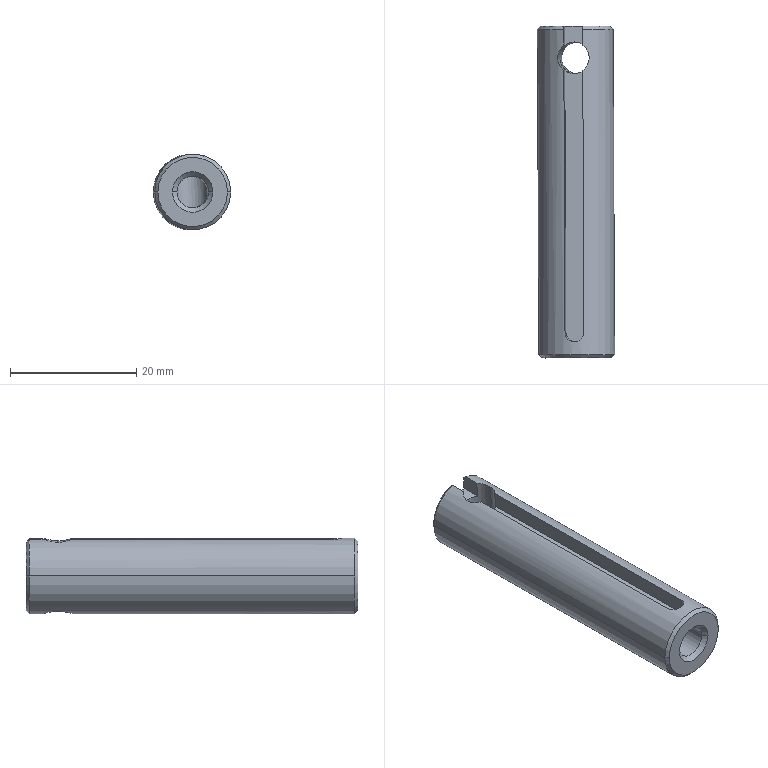Part | SolidWorks | features BaseBody 1 | 1 solid | 22 faces | box 12.224 x 52.547 x 12 mm | volume 4434 mm3 | plane 8 | cylinder 7 | cone 7 | commonest cylinder face diameters 5 x4 12 x2 3 x1
STEP:
#1=CARTESIAN_POINT('',(589.455,-135.542,110.117));
#2=VERTEX_POINT('',#1);
#3=CARTESIAN_POINT('',(585.292,-135.56,104.405));
#4=VERTEX_POINT('',#3);
#5=CARTESIAN_POINT('',(591.292,-135.534,104.405));
#6=DIRECTION('',(0.004352,-1.,-0.000000003));
#7=DIRECTION('',(1.,0.004352,0.));
#8=AXIS2_PLACEMENT_3D('',#5,#6,#7);
#9=CIRCLE('',#8,6.);
#10=EDGE_CURVE('',#2,#4,#9,.T.);
#11=ORIENTED_EDGE('',*,*,#10,.T.);
#12=CARTESIAN_POINT('',(585.516,-187.059,104.405));
#13=VERTEX_POINT('',#12);
#14=CARTESIAN_POINT('',(585.278,-132.435,104.405));
#15=DIRECTION('',(0.004352,-1.,-0.000000003));
#16=VECTOR('',#15,1000.);
#17=LINE('',#14,#16);
#18=EDGE_CURVE('',#4,#13,#17,.T.);
#19=ORIENTED_EDGE('',*,*,#18,.T.);
#20=CARTESIAN_POINT('',(597.516,-187.007,104.405));
#21=VERTEX_POINT('',#20);
#22=CARTESIAN_POINT('',(591.516,-187.033,104.405));
#23=DIRECTION('',(-0.004352,1.,0.000000003));
#24=DIRECTION('',(1.,0.004352,0.));
#25=AXIS2_PLACEMENT_3D('',#22,#23,#24);
#26=CIRCLE('',#25,6.);
#27=EDGE_CURVE('',#13,#21,#26,.T.);
#28=ORIENTED_EDGE('',*,*,#27,.T.);
#29=CARTESIAN_POINT('',(597.292,-135.507,104.405));
#30=VERTEX_POINT('',#29);
#31=CARTESIAN_POINT('',(597.278,-132.383,104.405));
#32=DIRECTION('',(0.004352,-1.,-0.000000003));
#33=VECTOR('',#32,1000.);
#34=LINE('',#31,#33);
#35=EDGE_CURVE('',#30,#21,#34,.T.);
#36=ORIENTED_EDGE('',*,*,#35,.F.);
#37=CARTESIAN_POINT('',(592.45,-135.529,110.292));
#38=VERTEX_POINT('',#37);
#39=CARTESIAN_POINT('',(591.292,-135.534,104.405));
#40=DIRECTION('',(0.004352,-1.,-0.000000003));
#41=DIRECTION('',(1.,0.004352,0.));
#42=AXIS2_PLACEMENT_3D('',#39,#40,#41);
#43=CIRCLE('',#42,6.);
#44=EDGE_CURVE('',#30,#38,#43,.T.);
#45=ORIENTED_EDGE('',*,*,#44,.T.);
#46=CARTESIAN_POINT('',(592.461,-138.029,110.292));
#47=VERTEX_POINT('',#46);
#48=CARTESIAN_POINT('',(592.436,-132.404,110.292));
#49=DIRECTION('',(0.004352,-1.,-0.000000003));
#50=VECTOR('',#49,1000.);
#51=LINE('',#48,#50);
#52=EDGE_CURVE('',#38,#47,#51,.T.);
#53=ORIENTED_EDGE('',*,*,#52,.T.);
#54=CARTESIAN_POINT('',(593.489,-140.035,109.996));
#55=VERTEX_POINT('',#54);
#56=CARTESIAN_POINT('',(592.461,-138.029,110.292));
#57=CARTESIAN_POINT('',(592.619,-138.145,110.261));
#58=CARTESIAN_POINT('',(592.761,-138.276,110.227));
#59=CARTESIAN_POINT('',(593.013,-138.569,110.158));
#60=CARTESIAN_POINT('',(593.124,-138.733,110.124));
#61=CARTESIAN_POINT('',(593.302,-139.077,110.065));
#62=CARTESIAN_POINT('',(593.371,-139.26,110.039));
#63=CARTESIAN_POINT('',(593.465,-139.644,110.005));
#64=CARTESIAN_POINT('',(593.489,-139.838,109.996));
#65=CARTESIAN_POINT('',(593.489,-140.035,109.996));
#66=B_SPLINE_CURVE_WITH_KNOTS('',3,(#56,#57,#58,#59,#60,#61,#62,#63,#64,#65),.UNSPECIFIED.,.F.,.F.,(4,2,2,2,4),(0.,0.000588,0.001176,0.001764,0.002352),.UNSPECIFIED.);
#67=EDGE_CURVE('',#47,#55,#66,.T.);
#68=ORIENTED_EDGE('',*,*,#67,.T.);
#69=CARTESIAN_POINT('',(592.478,-142.028,110.292));
#70=VERTEX_POINT('',#69);
#71=CARTESIAN_POINT('',(593.489,-140.035,109.996));
#72=CARTESIAN_POINT('',(593.489,-140.229,109.996));
#73=CARTESIAN_POINT('',(593.465,-140.426,110.006));
#74=CARTESIAN_POINT('',(593.373,-140.801,110.041));
#75=CARTESIAN_POINT('',(593.305,-140.984,110.066));
#76=CARTESIAN_POINT('',(593.042,-141.498,110.155));
#77=CARTESIAN_POINT('',(592.789,-141.796,110.231));
#78=CARTESIAN_POINT('',(592.478,-142.028,110.292));
#79=B_SPLINE_CURVE_WITH_KNOTS('',3,(#71,#72,#73,#74,#75,#76,#77,#78),.UNSPECIFIED.,.F.,.F.,(4,2,2,4),(0.002352,0.002933,0.003513,0.004674),.UNSPECIFIED.);
#80=EDGE_CURVE('',#55,#70,#79,.T.);
#81=ORIENTED_EDGE('',*,*,#80,.T.);
#82=CARTESIAN_POINT('',(592.659,-183.528,110.292));
#83=VERTEX_POINT('',#82);
#84=CARTESIAN_POINT('',(592.436,-132.404,110.292));
#85=DIRECTION('',(0.004352,-1.,-0.000000003));
#86=VECTOR('',#85,1000.);
#87=LINE('',#84,#86);
#88=EDGE_CURVE('',#70,#83,#87,.T.);
#89=ORIENTED_EDGE('',*,*,#88,.T.);
#90=CARTESIAN_POINT('',(589.664,-183.541,110.117));
#91=VERTEX_POINT('',#90);
#92=CARTESIAN_POINT('',(592.659,-183.528,110.292));
#93=CARTESIAN_POINT('',(592.659,-183.628,110.292));
#94=CARTESIAN_POINT('',(592.65,-183.725,110.294));
#95=CARTESIAN_POINT('',(592.612,-183.918,110.302));
#96=CARTESIAN_POINT('',(592.583,-184.013,110.307));
#97=CARTESIAN_POINT('',(592.508,-184.195,110.321));
#98=CARTESIAN_POINT('',(592.461,-184.281,110.328));
#99=CARTESIAN_POINT('',(592.352,-184.444,110.345));
#100=CARTESIAN_POINT('',(592.289,-184.521,110.354));
#101=CARTESIAN_POINT('',(592.081,-184.729,110.379));
#102=CARTESIAN_POINT('',(591.914,-184.841,110.394));
#103=CARTESIAN_POINT('',(591.553,-184.993,110.408));
#104=CARTESIAN_POINT('',(591.356,-185.034,110.406));
#105=CARTESIAN_POINT('',(591.058,-185.035,110.389));
#106=CARTESIAN_POINT('',(590.96,-185.026,110.381));
#107=CARTESIAN_POINT('',(590.769,-184.988,110.36));
#108=CARTESIAN_POINT('',(590.674,-184.96,110.348));
#109=CARTESIAN_POINT('',(590.493,-184.885,110.319));
#110=CARTESIAN_POINT('',(590.408,-184.839,110.304));
#111=CARTESIAN_POINT('',(590.246,-184.731,110.272));
#112=CARTESIAN_POINT('',(590.17,-184.669,110.255));
#113=CARTESIAN_POINT('',(589.965,-184.463,110.206));
#114=CARTESIAN_POINT('',(589.855,-184.297,110.174));
#115=CARTESIAN_POINT('',(589.705,-183.937,110.13));
#116=CARTESIAN_POINT('',(589.665,-183.74,110.117));
#117=CARTESIAN_POINT('',(589.664,-183.541,110.117));
#118=B_SPLINE_CURVE_WITH_KNOTS('',3,(#92,#93,#94,#95,#96,#97,#98,#99,#100,#101,#102,#103,#104,#105,#106,#107,#108,#109,#110,#111,#112,#113,#114,#115,#116,#117),.UNSPECIFIED.,.F.,.F.,(4,2,2,2,2,2,2,2,2,2,2,2,4),(0.,0.0002941,0.0005882,0.0008822,0.001176,0.001764,0.002353,0.002647,0.002941,0.003235,0.003529,0.004117,0.004705),.UNSPECIFIED.);
#119=EDGE_CURVE('',#83,#91,#118,.T.);
#120=ORIENTED_EDGE('',*,*,#119,.T.);
#121=CARTESIAN_POINT('',(589.484,-142.042,110.117));
#122=VERTEX_POINT('',#121);
#123=CARTESIAN_POINT('',(589.442,-132.417,110.117));
#124=DIRECTION('',(-0.004352,1.,0.000000003));
#125=VECTOR('',#124,1000.);
#126=LINE('',#123,#125);
#127=EDGE_CURVE('',#91,#122,#126,.T.);
#128=ORIENTED_EDGE('',*,*,#127,.T.);
#129=CARTESIAN_POINT('',(588.497,-140.035,109.704));
#130=VERTEX_POINT('',#129);
#131=CARTESIAN_POINT('',(589.484,-142.042,110.117));
#132=CARTESIAN_POINT('',(589.33,-141.925,110.068));
#133=CARTESIAN_POINT('',(589.193,-141.794,110.017));
#134=CARTESIAN_POINT('',(588.951,-141.501,109.92));
#135=CARTESIAN_POINT('',(588.845,-141.337,109.873));
#136=CARTESIAN_POINT('',(588.675,-140.993,109.793));
#137=CARTESIAN_POINT('',(588.609,-140.81,109.76));
#138=CARTESIAN_POINT('',(588.519,-140.426,109.715));
#139=CARTESIAN_POINT('',(588.497,-140.231,109.704));
#140=CARTESIAN_POINT('',(588.497,-140.035,109.704));
#141=B_SPLINE_CURVE_WITH_KNOTS('',3,(#131,#132,#133,#134,#135,#136,#137,#138,#139,#140),.UNSPECIFIED.,.F.,.F.,(4,2,2,2,4),(0.,0.000588,0.001176,0.001764,0.002352),.UNSPECIFIED.);
#142=EDGE_CURVE('',#122,#130,#141,.T.);
#143=ORIENTED_EDGE('',*,*,#142,.T.);
#144=CARTESIAN_POINT('',(589.466,-138.042,110.117));
#145=VERTEX_POINT('',#144);
#146=CARTESIAN_POINT('',(588.497,-140.035,109.704));
#147=CARTESIAN_POINT('',(588.497,-139.841,109.704));
#148=CARTESIAN_POINT('',(588.52,-139.644,109.717));
#149=CARTESIAN_POINT('',(588.606,-139.269,109.763));
#150=CARTESIAN_POINT('',(588.672,-139.086,109.796));
#151=CARTESIAN_POINT('',(588.923,-138.572,109.915));
#152=CARTESIAN_POINT('',(589.165,-138.274,110.02));
#153=CARTESIAN_POINT('',(589.466,-138.042,110.117));
#154=B_SPLINE_CURVE_WITH_KNOTS('',3,(#146,#147,#148,#149,#150,#151,#152,#153),.UNSPECIFIED.,.F.,.F.,(4,2,2,4),(0.002352,0.002933,0.003513,0.004674),.UNSPECIFIED.);
#155=EDGE_CURVE('',#130,#145,#154,.T.);
#156=ORIENTED_EDGE('',*,*,#155,.T.);
#157=CARTESIAN_POINT('',(589.442,-132.417,110.117));
#158=DIRECTION('',(-0.004352,1.,0.000000003));
#159=VECTOR('',#158,1000.);
#160=LINE('',#157,#159);
#161=EDGE_CURVE('',#145,#2,#160,.T.);
#162=ORIENTED_EDGE('',*,*,#161,.T.);
#163=EDGE_LOOP('',(#11,#19,#28,#36,#45,#53,#68,#81,#89,#120,#128,#143,#156,#162));
#164=FACE_OUTER_BOUND('',#163,.T.);
#165=CARTESIAN_POINT('',(591.278,-132.409,104.405));
#166=DIRECTION('',(0.004352,-1.,-0.000000003));
#167=DIRECTION('',(1.,0.004352,0.));
#168=AXIS2_PLACEMENT_3D('',#165,#166,#167);
#169=CYLINDRICAL_SURFACE('',#168,6.);
#170=ADVANCED_FACE('',(#164),#169,.T.);
#171=CARTESIAN_POINT('',(589.134,-140.032,98.814));
#172=VERTEX_POINT('',#171);
#173=CARTESIAN_POINT('',(594.126,-140.032,99.106));
#174=VERTEX_POINT('',#173);
#175=CARTESIAN_POINT('',(589.134,-140.032,98.814));
#176=CARTESIAN_POINT('',(589.134,-140.197,98.814));
#177=CARTESIAN_POINT('',(589.151,-140.365,98.808));
#178=CARTESIAN_POINT('',(589.218,-140.687,98.783));
#179=CARTESIAN_POINT('',(589.267,-140.844,98.765));
#180=CARTESIAN_POINT('',(589.397,-141.149,98.72));
#181=CARTESIAN_POINT('',(589.476,-141.292,98.693));
#182=CARTESIAN_POINT('',(589.66,-141.56,98.638));
#183=CARTESIAN_POINT('',(589.767,-141.687,98.608));
#184=CARTESIAN_POINT('',(589.999,-141.915,98.551));
#185=CARTESIAN_POINT('',(590.125,-142.018,98.523));
#186=CARTESIAN_POINT('',(590.399,-142.199,98.475));
#187=CARTESIAN_POINT('',(590.546,-142.277,98.453));
#188=CARTESIAN_POINT('',(591.,-142.465,98.406));
#189=CARTESIAN_POINT('',(591.332,-142.533,98.396));
#190=CARTESIAN_POINT('',(591.833,-142.532,98.424));
#191=CARTESIAN_POINT('',(591.996,-142.515,98.441));
#192=CARTESIAN_POINT('',(592.316,-142.45,98.486));
#193=CARTESIAN_POINT('',(592.474,-142.4,98.515));
#194=CARTESIAN_POINT('',(592.773,-142.274,98.581));
#195=CARTESIAN_POINT('',(592.914,-142.197,98.619));
#196=CARTESIAN_POINT('',(593.179,-142.015,98.699));
#197=CARTESIAN_POINT('',(593.303,-141.911,98.741));
#198=CARTESIAN_POINT('',(593.637,-141.568,98.866));
#199=CARTESIAN_POINT('',(593.817,-141.293,98.949));
#200=CARTESIAN_POINT('',(594.,-140.843,99.039));
#201=CARTESIAN_POINT('',(594.047,-140.684,99.063));
#202=CARTESIAN_POINT('',(594.11,-140.361,99.097));
#203=CARTESIAN_POINT('',(594.126,-140.197,99.106));
#204=CARTESIAN_POINT('',(594.126,-140.032,99.106));
#205=B_SPLINE_CURVE_WITH_KNOTS('',3,(#175,#176,#177,#178,#179,#180,#181,#182,#183,#184,#185,#186,#187,#188,#189,#190,#191,#192,#193,#194,#195,#196,#197,#198,#199,#200,#201,#202,#203,#204),.UNSPECIFIED.,.F.,.F.,(4,2,2,2,2,2,2,2,2,2,2,2,2,2,4),(0.01185,0.01234,0.01283,0.01333,0.01382,0.01432,0.01481,0.0158,0.01629,0.01679,0.01728,0.01777,0.01876,0.01926,0.01975),.UNSPECIFIED.);
#206=EDGE_CURVE('',#172,#174,#205,.T.);
#207=ORIENTED_EDGE('',*,*,#206,.F.);
#208=CARTESIAN_POINT('',(588.395,-140.035,111.447));
#209=DIRECTION('',(-0.05839,-0.0002541,0.9983));
#210=VECTOR('',#209,1000.);
#211=LINE('',#208,#210);
#212=EDGE_CURVE('',#172,#130,#211,.T.);
#213=ORIENTED_EDGE('',*,*,#212,.T.);
#214=ORIENTED_EDGE('',*,*,#142,.F.);
#215=CARTESIAN_POINT('',(589.636,-142.041,107.512));
#216=VERTEX_POINT('',#215);
#217=CARTESIAN_POINT('',(589.402,-142.042,111.505));
#218=DIRECTION('',(-0.05839,-0.0002541,0.9983));
#219=VECTOR('',#218,1000.);
#220=LINE('',#217,#219);
#221=EDGE_CURVE('',#216,#122,#220,.T.);
#222=ORIENTED_EDGE('',*,*,#221,.F.);
#223=CARTESIAN_POINT('',(592.631,-142.028,107.687));
#224=VERTEX_POINT('',#223);
#225=CARTESIAN_POINT('',(591.125,-140.034,107.6));
#226=DIRECTION('',(0.05839,0.0002541,-0.9983));
#227=DIRECTION('',(0.9983,0.,0.05839));
#228=AXIS2_PLACEMENT_3D('',#225,#226,#227);
#229=CIRCLE('',#228,2.5);
#230=EDGE_CURVE('',#224,#216,#229,.T.);
#231=ORIENTED_EDGE('',*,*,#230,.F.);
#232=CARTESIAN_POINT('',(592.397,-142.029,111.68));
#233=DIRECTION('',(0.05839,0.0002541,-0.9983));
#234=VECTOR('',#233,1000.);
#235=LINE('',#232,#234);
#236=EDGE_CURVE('',#70,#224,#235,.T.);
#237=ORIENTED_EDGE('',*,*,#236,.F.);
#238=ORIENTED_EDGE('',*,*,#80,.F.);
#239=CARTESIAN_POINT('',(593.807,-140.034,104.562));
#240=VERTEX_POINT('',#239);
#241=CARTESIAN_POINT('',(593.387,-140.035,111.739));
#242=DIRECTION('',(-0.05839,-0.0002541,0.9983));
#243=VECTOR('',#242,1000.);
#244=LINE('',#241,#243);
#245=EDGE_CURVE('',#240,#55,#244,.T.);
#246=ORIENTED_EDGE('',*,*,#245,.F.);
#247=CARTESIAN_POINT('',(588.812,-140.19,104.405));
#248=VERTEX_POINT('',#247);
#249=CARTESIAN_POINT('',(588.812,-140.19,104.405));
#250=CARTESIAN_POINT('',(588.833,-144.885,109.107));
#251=CARTESIAN_POINT('',(593.532,-144.737,109.255));
#252=CARTESIAN_POINT('',(593.807,-140.034,104.562));
#253=(BOUNDED_CURVE()B_SPLINE_CURVE(3,(#249,#250,#251,#252),.UNSPECIFIED.,.F.,.F.)B_SPLINE_CURVE_WITH_KNOTS((4,4),(4.771,7.85),.UNSPECIFIED.)CURVE()GEOMETRIC_REPRESENTATION_ITEM()RATIONAL_B_SPLINE_CURVE((1.,0.3543,0.3543,1.))REPRESENTATION_ITEM(''));
#254=EDGE_CURVE('',#248,#240,#253,.T.);
#255=ORIENTED_EDGE('',*,*,#254,.F.);
#256=CARTESIAN_POINT('',(588.816,-140.044,104.259));
#257=VERTEX_POINT('',#256);
#258=CARTESIAN_POINT('',(588.816,-140.044,104.259));
#259=CARTESIAN_POINT('',(588.813,-140.093,104.308));
#260=CARTESIAN_POINT('',(588.812,-140.142,104.356));
#261=CARTESIAN_POINT('',(588.812,-140.19,104.405));
#262=(BOUNDED_CURVE()B_SPLINE_CURVE(3,(#258,#259,#260,#261),.UNSPECIFIED.,.F.,.F.)B_SPLINE_CURVE_WITH_KNOTS((4,4),(4.712,4.771),.UNSPECIFIED.)CURVE()GEOMETRIC_REPRESENTATION_ITEM()RATIONAL_B_SPLINE_CURVE((1.,0.9997,0.9997,1.))REPRESENTATION_ITEM(''));
#263=EDGE_CURVE('',#257,#248,#262,.T.);
#264=ORIENTED_EDGE('',*,*,#263,.F.);
#265=CARTESIAN_POINT('',(593.812,-140.169,104.405));
#266=VERTEX_POINT('',#265);
#267=CARTESIAN_POINT('',(593.812,-140.169,104.405));
#268=CARTESIAN_POINT('',(593.833,-144.883,99.683));
#269=CARTESIAN_POINT('',(589.112,-144.765,99.545));
#270=CARTESIAN_POINT('',(588.816,-140.044,104.259));
#271=(BOUNDED_CURVE()B_SPLINE_CURVE(3,(#267,#268,#269,#270),.UNSPECIFIED.,.F.,.F.)B_SPLINE_CURVE_WITH_KNOTS((4,4),(4.771,7.854),.UNSPECIFIED.)CURVE()GEOMETRIC_REPRESENTATION_ITEM()RATIONAL_B_SPLINE_CURVE((1.,0.3528,0.3528,1.))REPRESENTATION_ITEM(''));
#272=EDGE_CURVE('',#266,#257,#271,.T.);
#273=ORIENTED_EDGE('',*,*,#272,.F.);
#274=CARTESIAN_POINT('',(593.808,-140.034,104.54));
#275=VERTEX_POINT('',#274);
#276=CARTESIAN_POINT('',(593.808,-140.034,104.54));
#277=CARTESIAN_POINT('',(593.81,-140.079,104.495));
#278=CARTESIAN_POINT('',(593.812,-140.124,104.45));
#279=CARTESIAN_POINT('',(593.812,-140.169,104.405));
#280=(BOUNDED_CURVE()B_SPLINE_CURVE(3,(#276,#277,#278,#279),.UNSPECIFIED.,.F.,.F.)B_SPLINE_CURVE_WITH_KNOTS((4,4),(4.717,4.771),.UNSPECIFIED.)CURVE()GEOMETRIC_REPRESENTATION_ITEM()RATIONAL_B_SPLINE_CURVE((1.,0.9998,0.9998,1.))REPRESENTATION_ITEM(''));
#281=EDGE_CURVE('',#275,#266,#280,.T.);
#282=ORIENTED_EDGE('',*,*,#281,.F.);
#283=CARTESIAN_POINT('',(593.387,-140.035,111.739));
#284=DIRECTION('',(-0.05839,-0.0002541,0.9983));
#285=VECTOR('',#284,1000.);
#286=LINE('',#283,#285);
#287=EDGE_CURVE('',#174,#275,#286,.T.);
#288=ORIENTED_EDGE('',*,*,#287,.F.);
#289=EDGE_LOOP('',(#207,#213,#214,#222,#231,#237,#238,#246,#255,#264,#273,#282,#288));
#290=FACE_OUTER_BOUND('',#289,.T.);
#291=CARTESIAN_POINT('',(590.891,-140.035,111.593));
#292=DIRECTION('',(-0.05839,-0.0002541,0.9983));
#293=DIRECTION('',(0.9983,0.,0.05839));
#294=AXIS2_PLACEMENT_3D('',#291,#292,#293);
#295=CYLINDRICAL_SURFACE('',#294,2.5);
#296=ADVANCED_FACE('',(#290),#295,.F.);
#297=CARTESIAN_POINT('',(586.018,-187.557,104.405));
#298=VERTEX_POINT('',#297);
#299=CARTESIAN_POINT('',(597.018,-187.509,104.405));
#300=VERTEX_POINT('',#299);
#301=CARTESIAN_POINT('',(591.518,-187.533,104.405));
#302=DIRECTION('',(-0.004352,1.,0.000000003));
#303=DIRECTION('',(-1.,-0.004352,0.));
#304=AXIS2_PLACEMENT_3D('',#301,#302,#303);
#305=CIRCLE('',#304,5.5);
#306=EDGE_CURVE('',#298,#300,#305,.T.);
#307=ORIENTED_EDGE('',*,*,#306,.T.);
#308=CARTESIAN_POINT('',(597.516,-187.007,104.405));
#309=DIRECTION('',(0.704,0.7102,0.000000002));
#310=VECTOR('',#309,1000.);
#311=LINE('',#308,#310);
#312=EDGE_CURVE('',#300,#21,#311,.T.);
#313=ORIENTED_EDGE('',*,*,#312,.T.);
#314=ORIENTED_EDGE('',*,*,#27,.F.);
#315=CARTESIAN_POINT('',(585.516,-187.059,104.405));
#316=DIRECTION('',(-0.7102,0.704,0.000000002));
#317=VECTOR('',#316,1000.);
#318=LINE('',#315,#317);
#319=EDGE_CURVE('',#298,#13,#318,.T.);
#320=ORIENTED_EDGE('',*,*,#319,.F.);
#321=EDGE_LOOP('',(#307,#313,#314,#320));
#322=FACE_OUTER_BOUND('',#321,.T.);
#323=CARTESIAN_POINT('',(591.516,-187.033,104.405));
#324=DIRECTION('',(-0.004352,1.,0.000000003));
#325=DIRECTION('',(-1.,-0.004352,0.));
#326=AXIS2_PLACEMENT_3D('',#323,#324,#325);
#327=CONICAL_SURFACE('',#326,6.,0.7854);
#328=ADVANCED_FACE('',(#322),#327,.T.);
#329=CARTESIAN_POINT('',(589.483,-135.041,109.6));
#330=VERTEX_POINT('',#329);
#331=CARTESIAN_POINT('',(585.79,-135.058,104.405));
#332=VERTEX_POINT('',#331);
#333=CARTESIAN_POINT('',(591.29,-135.034,104.405));
#334=DIRECTION('',(0.004352,-1.,-0.000000003));
#335=DIRECTION('',(1.,0.004352,0.));
#336=AXIS2_PLACEMENT_3D('',#333,#334,#335);
#337=CIRCLE('',#336,5.5);
#338=EDGE_CURVE('',#330,#332,#337,.T.);
#339=ORIENTED_EDGE('',*,*,#338,.T.);
#340=CARTESIAN_POINT('',(585.292,-135.56,104.405));
#341=DIRECTION('',(-0.704,-0.7102,-0.000000002));
#342=VECTOR('',#341,1000.);
#343=LINE('',#340,#342);
#344=EDGE_CURVE('',#332,#4,#343,.T.);
#345=ORIENTED_EDGE('',*,*,#344,.T.);
#346=ORIENTED_EDGE('',*,*,#10,.F.);
#347=CARTESIAN_POINT('',(589.455,-135.542,110.117));
#348=CARTESIAN_POINT('',(589.465,-135.375,109.945));
#349=CARTESIAN_POINT('',(589.474,-135.208,109.772));
#350=CARTESIAN_POINT('',(589.483,-135.041,109.6));
#351=B_SPLINE_CURVE_WITH_KNOTS('',3,(#347,#348,#349,#350),.UNSPECIFIED.,.F.,.F.,(4,4),(0.,0.0007199),.UNSPECIFIED.);
#352=EDGE_CURVE('',#2,#330,#351,.T.);
#353=ORIENTED_EDGE('',*,*,#352,.T.);
#354=EDGE_LOOP('',(#339,#345,#346,#353));
#355=FACE_OUTER_BOUND('',#354,.T.);
#356=CARTESIAN_POINT('',(591.292,-135.534,104.405));
#357=DIRECTION('',(0.004352,-1.,-0.000000003));
#358=DIRECTION('',(1.,0.004352,0.));
#359=AXIS2_PLACEMENT_3D('',#356,#357,#358);
#360=CONICAL_SURFACE('',#359,6.,0.7854);
#361=ADVANCED_FACE('',(#355),#360,.T.);
#362=ORIENTED_EDGE('',*,*,#344,.F.);
#363=CARTESIAN_POINT('',(596.79,-135.01,104.405));
#364=VERTEX_POINT('',#363);
#365=CARTESIAN_POINT('',(591.29,-135.034,104.405));
#366=DIRECTION('',(0.004352,-1.,-0.000000003));
#367=DIRECTION('',(1.,0.004352,0.));
#368=AXIS2_PLACEMENT_3D('',#365,#366,#367);
#369=CIRCLE('',#368,5.5);
#370=EDGE_CURVE('',#332,#364,#369,.T.);
#371=ORIENTED_EDGE('',*,*,#370,.T.);
#372=CARTESIAN_POINT('',(597.292,-135.507,104.405));
#373=DIRECTION('',(0.7102,-0.704,-0.000000002));
#374=VECTOR('',#373,1000.);
#375=LINE('',#372,#374);
#376=EDGE_CURVE('',#364,#30,#375,.T.);
#377=ORIENTED_EDGE('',*,*,#376,.T.);
#378=CARTESIAN_POINT('',(591.292,-135.534,104.405));
#379=DIRECTION('',(0.004352,-1.,-0.000000003));
#380=DIRECTION('',(1.,0.004352,0.));
#381=AXIS2_PLACEMENT_3D('',#378,#379,#380);
#382=CIRCLE('',#381,6.);
#383=EDGE_CURVE('',#4,#30,#382,.T.);
#384=ORIENTED_EDGE('',*,*,#383,.F.);
#385=EDGE_LOOP('',(#362,#371,#377,#384));
#386=FACE_OUTER_BOUND('',#385,.T.);
#387=CARTESIAN_POINT('',(591.292,-135.534,104.405));
#388=DIRECTION('',(0.004352,-1.,-0.000000003));
#389=DIRECTION('',(1.,0.004352,0.));
#390=AXIS2_PLACEMENT_3D('',#387,#388,#389);
#391=CONICAL_SURFACE('',#390,6.,0.7854);
#392=ADVANCED_FACE('',(#386),#391,.T.);
#393=ORIENTED_EDGE('',*,*,#263,.T.);
#394=CARTESIAN_POINT('',(589.015,-186.844,104.405));
#395=VERTEX_POINT('',#394);
#396=CARTESIAN_POINT('',(588.795,-136.154,104.405));
#397=DIRECTION('',(0.004352,-1.,-0.000000003));
#398=VECTOR('',#397,1000.);
#399=LINE('',#396,#398);
#400=EDGE_CURVE('',#248,#395,#399,.T.);
#401=ORIENTED_EDGE('',*,*,#400,.T.);
#402=CARTESIAN_POINT('',(594.015,-186.822,104.405));
#403=VERTEX_POINT('',#402);
#404=CARTESIAN_POINT('',(591.515,-186.833,104.405));
#405=DIRECTION('',(-0.004352,1.,0.000000003));
#406=DIRECTION('',(1.,0.004352,0.));
#407=AXIS2_PLACEMENT_3D('',#404,#405,#406);
#408=CIRCLE('',#407,2.5);
#409=EDGE_CURVE('',#403,#395,#408,.T.);
#410=ORIENTED_EDGE('',*,*,#409,.F.);
#411=CARTESIAN_POINT('',(593.795,-136.132,104.405));
#412=DIRECTION('',(0.004352,-1.,-0.000000003));
#413=VECTOR('',#412,1000.);
#414=LINE('',#411,#413);
#415=EDGE_CURVE('',#266,#403,#414,.T.);
#416=ORIENTED_EDGE('',*,*,#415,.F.);
#417=ORIENTED_EDGE('',*,*,#272,.T.);
#418=EDGE_LOOP('',(#393,#401,#410,#416,#417));
#419=FACE_OUTER_BOUND('',#418,.T.);
#420=CARTESIAN_POINT('',(591.295,-136.143,104.405));
#421=DIRECTION('',(0.004352,-1.,-0.000000003));
#422=DIRECTION('',(1.,0.004352,0.));
#423=AXIS2_PLACEMENT_3D('',#420,#421,#422);
#424=CYLINDRICAL_SURFACE('',#423,2.5);
#425=ADVANCED_FACE('',(#419),#424,.F.);
#426=ORIENTED_EDGE('',*,*,#409,.T.);
#427=CARTESIAN_POINT('',(588.318,-187.547,104.405));
#428=VERTEX_POINT('',#427);
#429=CARTESIAN_POINT('',(588.318,-187.547,104.405));
#430=DIRECTION('',(-0.704,-0.7102,-0.000000002));
#431=VECTOR('',#430,1000.);
#432=LINE('',#429,#431);
#433=EDGE_CURVE('',#395,#428,#432,.T.);
#434=ORIENTED_EDGE('',*,*,#433,.T.);
#435=CARTESIAN_POINT('',(594.718,-187.519,104.405));
#436=VERTEX_POINT('',#435);
#437=CARTESIAN_POINT('',(591.518,-187.533,104.405));
#438=DIRECTION('',(-0.004352,1.,0.000000003));
#439=DIRECTION('',(1.,0.004352,0.));
#440=AXIS2_PLACEMENT_3D('',#437,#438,#439);
#441=CIRCLE('',#440,3.2);
#442=EDGE_CURVE('',#436,#428,#441,.T.);
#443=ORIENTED_EDGE('',*,*,#442,.F.);
#444=CARTESIAN_POINT('',(594.718,-187.519,104.405));
#445=DIRECTION('',(0.7102,-0.704,-0.000000002));
#446=VECTOR('',#445,1000.);
#447=LINE('',#444,#446);
#448=EDGE_CURVE('',#403,#436,#447,.T.);
#449=ORIENTED_EDGE('',*,*,#448,.F.);
#450=EDGE_LOOP('',(#426,#434,#443,#449));
#451=FACE_OUTER_BOUND('',#450,.T.);
#452=CARTESIAN_POINT('',(591.518,-187.533,104.405));
#453=DIRECTION('',(0.004352,-1.,-0.000000003));
#454=DIRECTION('',(1.,0.004352,0.));
#455=AXIS2_PLACEMENT_3D('',#452,#453,#454);
#456=CONICAL_SURFACE('',#455,3.2,0.7854);
#457=ADVANCED_FACE('',(#451),#456,.F.);
#458=ORIENTED_EDGE('',*,*,#18,.F.);
#459=ORIENTED_EDGE('',*,*,#383,.T.);
#460=ORIENTED_EDGE('',*,*,#35,.T.);
#461=CARTESIAN_POINT('',(591.516,-187.033,104.405));
#462=DIRECTION('',(-0.004352,1.,0.000000003));
#463=DIRECTION('',(1.,0.004352,0.));
#464=AXIS2_PLACEMENT_3D('',#461,#462,#463);
#465=CIRCLE('',#464,6.);
#466=EDGE_CURVE('',#21,#13,#465,.T.);
#467=ORIENTED_EDGE('',*,*,#466,.T.);
#468=EDGE_LOOP('',(#458,#459,#460,#467));
#469=FACE_OUTER_BOUND('',#468,.T.);
#470=CARTESIAN_POINT('',(594.126,-140.032,99.106));
#471=CARTESIAN_POINT('',(594.126,-139.867,99.106));
#472=CARTESIAN_POINT('',(594.109,-139.699,99.098));
#473=CARTESIAN_POINT('',(594.046,-139.377,99.066));
#474=CARTESIAN_POINT('',(593.999,-139.22,99.042));
#475=CARTESIAN_POINT('',(593.876,-138.916,98.982));
#476=CARTESIAN_POINT('',(593.8,-138.773,98.947));
#477=CARTESIAN_POINT('',(593.624,-138.504,98.871));
#478=CARTESIAN_POINT('',(593.522,-138.377,98.829));
#479=CARTESIAN_POINT('',(593.298,-138.149,98.745));
#480=CARTESIAN_POINT('',(593.176,-138.047,98.703));
#481=CARTESIAN_POINT('',(592.91,-137.866,98.623));
#482=CARTESIAN_POINT('',(592.767,-137.787,98.585));
#483=CARTESIAN_POINT('',(592.321,-137.6,98.485));
#484=CARTESIAN_POINT('',(591.993,-137.532,98.436));
#485=CARTESIAN_POINT('',(591.492,-137.532,98.406));
#486=CARTESIAN_POINT('',(591.328,-137.549,98.403));
#487=CARTESIAN_POINT('',(591.005,-137.614,98.41));
#488=CARTESIAN_POINT('',(590.844,-137.663,98.42));
#489=CARTESIAN_POINT('',(590.54,-137.79,98.452));
#490=CARTESIAN_POINT('',(590.396,-137.867,98.472));
#491=CARTESIAN_POINT('',(590.122,-138.049,98.521));
#492=CARTESIAN_POINT('',(589.994,-138.153,98.548));
#493=CARTESIAN_POINT('',(589.648,-138.495,98.633));
#494=CARTESIAN_POINT('',(589.459,-138.771,98.695));
#495=CARTESIAN_POINT('',(589.267,-139.221,98.762));
#496=CARTESIAN_POINT('',(589.217,-139.38,98.781));
#497=CARTESIAN_POINT('',(589.151,-139.704,98.807));
#498=CARTESIAN_POINT('',(589.134,-139.867,98.814));
#499=CARTESIAN_POINT('',(589.134,-140.032,98.814));
#500=B_SPLINE_CURVE_WITH_KNOTS('',3,(#470,#471,#472,#473,#474,#475,#476,#477,#478,#479,#480,#481,#482,#483,#484,#485,#486,#487,#488,#489,#490,#491,#492,#493,#494,#495,#496,#497,#498,#499),.UNSPECIFIED.,.F.,.F.,(4,2,2,2,2,2,2,2,2,2,2,2,2,2,4),(0.003944,0.004438,0.004932,0.005426,0.00592,0.006414,0.006908,0.007896,0.00839,0.008883,0.009377,0.009871,0.01086,0.01135,0.01185),.UNSPECIFIED.);
#501=EDGE_CURVE('',#174,#172,#500,.T.);
#502=ORIENTED_EDGE('',*,*,#501,.T.);
#503=ORIENTED_EDGE('',*,*,#206,.T.);
#504=EDGE_LOOP('',(#502,#503));
#505=FACE_BOUND('',#504,.T.);
#506=CARTESIAN_POINT('',(591.278,-132.409,104.405));
#507=DIRECTION('',(0.004352,-1.,-0.000000003));
#508=DIRECTION('',(1.,0.004352,0.));
#509=AXIS2_PLACEMENT_3D('',#506,#507,#508);
#510=CYLINDRICAL_SURFACE('',#509,6.);
#511=ADVANCED_FACE('',(#469,#505),#510,.T.);
#512=ORIENTED_EDGE('',*,*,#212,.F.);
#513=ORIENTED_EDGE('',*,*,#501,.F.);
#514=ORIENTED_EDGE('',*,*,#287,.T.);
#515=CARTESIAN_POINT('',(593.807,-140.023,104.551));
#516=VERTEX_POINT('',#515);
#517=CARTESIAN_POINT('',(593.807,-140.023,104.551));
#518=CARTESIAN_POINT('',(593.807,-140.026,104.547));
#519=CARTESIAN_POINT('',(593.808,-140.03,104.544));
#520=CARTESIAN_POINT('',(593.808,-140.034,104.54));
#521=(BOUNDED_CURVE()B_SPLINE_CURVE(3,(#517,#518,#519,#520),.UNSPECIFIED.,.F.,.F.)B_SPLINE_CURVE_WITH_KNOTS((4,4),(4.712,4.717),.UNSPECIFIED.)CURVE()GEOMETRIC_REPRESENTATION_ITEM()RATIONAL_B_SPLINE_CURVE((1.,1.,1.,1.))REPRESENTATION_ITEM(''));
#522=EDGE_CURVE('',#516,#275,#521,.T.);
#523=ORIENTED_EDGE('',*,*,#522,.F.);
#524=CARTESIAN_POINT('',(593.807,-140.034,104.562));
#525=CARTESIAN_POINT('',(593.807,-140.03,104.558));
#526=CARTESIAN_POINT('',(593.807,-140.026,104.555));
#527=CARTESIAN_POINT('',(593.807,-140.023,104.551));
#528=(BOUNDED_CURVE()B_SPLINE_CURVE(3,(#524,#525,#526,#527),.UNSPECIFIED.,.F.,.F.)B_SPLINE_CURVE_WITH_KNOTS((4,4),(1.566,1.571),.UNSPECIFIED.)CURVE()GEOMETRIC_REPRESENTATION_ITEM()RATIONAL_B_SPLINE_CURVE((1.,1.,1.,1.))REPRESENTATION_ITEM(''));
#529=EDGE_CURVE('',#240,#516,#528,.T.);
#530=ORIENTED_EDGE('',*,*,#529,.F.);
#531=ORIENTED_EDGE('',*,*,#245,.T.);
#532=ORIENTED_EDGE('',*,*,#67,.F.);
#533=CARTESIAN_POINT('',(592.613,-138.028,107.687));
#534=VERTEX_POINT('',#533);
#535=CARTESIAN_POINT('',(592.38,-138.029,111.68));
#536=DIRECTION('',(-0.05839,-0.0002541,0.9983));
#537=VECTOR('',#536,1000.);
#538=LINE('',#535,#537);
#539=EDGE_CURVE('',#534,#47,#538,.T.);
#540=ORIENTED_EDGE('',*,*,#539,.F.);
#541=CARTESIAN_POINT('',(589.618,-138.041,107.512));
#542=VERTEX_POINT('',#541);
#543=CARTESIAN_POINT('',(591.125,-140.034,107.6));
#544=DIRECTION('',(0.05839,0.0002541,-0.9983));
#545=DIRECTION('',(0.9983,0.,0.05839));
#546=AXIS2_PLACEMENT_3D('',#543,#544,#545);
#547=CIRCLE('',#546,2.5);
#548=EDGE_CURVE('',#542,#534,#547,.T.);
#549=ORIENTED_EDGE('',*,*,#548,.F.);
#550=CARTESIAN_POINT('',(589.385,-138.042,111.505));
#551=DIRECTION('',(0.05839,0.0002541,-0.9983));
#552=VECTOR('',#551,1000.);
#553=LINE('',#550,#552);
#554=EDGE_CURVE('',#145,#542,#553,.T.);
#555=ORIENTED_EDGE('',*,*,#554,.F.);
#556=ORIENTED_EDGE('',*,*,#155,.F.);
#557=EDGE_LOOP('',(#512,#513,#514,#523,#530,#531,#532,#540,#549,#555,#556));
#558=FACE_OUTER_BOUND('',#557,.T.);
#559=CARTESIAN_POINT('',(590.891,-140.035,111.593));
#560=DIRECTION('',(-0.05839,-0.0002541,0.9983));
#561=DIRECTION('',(0.9983,0.,0.05839));
#562=AXIS2_PLACEMENT_3D('',#559,#560,#561);
#563=CYLINDRICAL_SURFACE('',#562,2.5);
#564=ADVANCED_FACE('',(#558),#563,.F.);
#565=ORIENTED_EDGE('',*,*,#312,.F.);
#566=CARTESIAN_POINT('',(591.518,-187.533,104.405));
#567=DIRECTION('',(-0.004352,1.,0.000000003));
#568=DIRECTION('',(-1.,-0.004352,0.));
#569=AXIS2_PLACEMENT_3D('',#566,#567,#568);
#570=CIRCLE('',#569,5.5);
#571=EDGE_CURVE('',#300,#298,#570,.T.);
#572=ORIENTED_EDGE('',*,*,#571,.T.);
#573=ORIENTED_EDGE('',*,*,#319,.T.);
#574=ORIENTED_EDGE('',*,*,#466,.F.);
#575=EDGE_LOOP('',(#565,#572,#573,#574));
#576=FACE_OUTER_BOUND('',#575,.T.);
#577=CARTESIAN_POINT('',(591.516,-187.033,104.405));
#578=DIRECTION('',(-0.004352,1.,0.000000003));
#579=DIRECTION('',(-1.,-0.004352,0.));
#580=AXIS2_PLACEMENT_3D('',#577,#578,#579);
#581=CONICAL_SURFACE('',#580,6.,0.7854);
#582=ADVANCED_FACE('',(#576),#581,.T.);
#583=ORIENTED_EDGE('',*,*,#119,.F.);
#584=CARTESIAN_POINT('',(592.811,-183.527,107.687));
#585=VERTEX_POINT('',#584);
#586=CARTESIAN_POINT('',(592.816,-183.527,107.602));
#587=DIRECTION('',(-0.05839,-0.0002541,0.9983));
#588=VECTOR('',#587,1000.);
#589=LINE('',#586,#588);
#590=EDGE_CURVE('',#585,#83,#589,.T.);
#591=ORIENTED_EDGE('',*,*,#590,.F.);
#592=CARTESIAN_POINT('',(589.817,-183.54,107.512));
#593=VERTEX_POINT('',#592);
#594=CARTESIAN_POINT('',(591.314,-183.534,107.6));
#595=DIRECTION('',(-0.05839,-0.0002541,0.9983));
#596=DIRECTION('',(-0.9983,0.,-0.05839));
#597=AXIS2_PLACEMENT_3D('',#594,#595,#596);
#598=CIRCLE('',#597,1.5);
#599=EDGE_CURVE('',#593,#585,#598,.T.);
#600=ORIENTED_EDGE('',*,*,#599,.F.);
#601=CARTESIAN_POINT('',(589.821,-183.54,107.427));
#602=DIRECTION('',(0.05839,0.0002541,-0.9983));
#603=VECTOR('',#602,1000.);
#604=LINE('',#601,#603);
#605=EDGE_CURVE('',#91,#593,#604,.T.);
#606=ORIENTED_EDGE('',*,*,#605,.F.);
#607=EDGE_LOOP('',(#583,#591,#600,#606));
#608=FACE_OUTER_BOUND('',#607,.T.);
#609=CARTESIAN_POINT('',(591.319,-183.534,107.515));
#610=DIRECTION('',(0.05839,0.0002541,-0.9983));
#611=DIRECTION('',(-0.9983,0.,-0.05839));
#612=AXIS2_PLACEMENT_3D('',#609,#610,#611);
#613=CYLINDRICAL_SURFACE('',#612,1.5);
#614=ADVANCED_FACE('',(#608),#613,.F.);
#615=ORIENTED_EDGE('',*,*,#236,.T.);
#616=CARTESIAN_POINT('',(592.811,-183.527,107.687));
#617=DIRECTION('',(-0.004352,1.,0.000000003));
#618=VECTOR('',#617,1000.);
#619=LINE('',#616,#618);
#620=EDGE_CURVE('',#585,#224,#619,.T.);
#621=ORIENTED_EDGE('',*,*,#620,.F.);
#622=ORIENTED_EDGE('',*,*,#590,.T.);
#623=ORIENTED_EDGE('',*,*,#88,.F.);
#624=EDGE_LOOP('',(#615,#621,#622,#623));
#625=FACE_OUTER_BOUND('',#624,.T.);
#626=CARTESIAN_POINT('',(592.448,-135.029,110.292));
#627=DIRECTION('',(0.9983,0.004345,0.05839));
#628=DIRECTION('',(0.0584,0.,-0.9983));
#629=AXIS2_PLACEMENT_3D('',#626,#627,#628);
#630=PLANE('',#629);
#631=ADVANCED_FACE('',(#625),#630,.F.);
#632=ORIENTED_EDGE('',*,*,#539,.T.);
#633=ORIENTED_EDGE('',*,*,#52,.F.);
#634=CARTESIAN_POINT('',(592.478,-135.028,109.775));
#635=VERTEX_POINT('',#634);
#636=CARTESIAN_POINT('',(592.478,-135.028,109.775));
#637=CARTESIAN_POINT('',(592.469,-135.195,109.948));
#638=CARTESIAN_POINT('',(592.459,-135.362,110.12));
#639=CARTESIAN_POINT('',(592.45,-135.529,110.292));
#640=B_SPLINE_CURVE_WITH_KNOTS('',3,(#636,#637,#638,#639),.UNSPECIFIED.,.F.,.F.,(4,4),(0.,0.0007199),.UNSPECIFIED.);
#641=EDGE_CURVE('',#635,#38,#640,.T.);
#642=ORIENTED_EDGE('',*,*,#641,.F.);
#643=CARTESIAN_POINT('',(592.6,-135.028,107.687));
#644=VERTEX_POINT('',#643);
#645=CARTESIAN_POINT('',(592.6,-135.028,107.687));
#646=DIRECTION('',(-0.05839,-0.0002541,0.9983));
#647=VECTOR('',#646,1000.);
#648=LINE('',#645,#647);
#649=EDGE_CURVE('',#644,#635,#648,.T.);
#650=ORIENTED_EDGE('',*,*,#649,.F.);
#651=CARTESIAN_POINT('',(592.613,-138.028,107.687));
#652=DIRECTION('',(-0.004352,1.,0.000000003));
#653=VECTOR('',#652,1000.);
#654=LINE('',#651,#653);
#655=EDGE_CURVE('',#534,#644,#654,.T.);
#656=ORIENTED_EDGE('',*,*,#655,.F.);
#657=EDGE_LOOP('',(#632,#633,#642,#650,#656));
#658=FACE_OUTER_BOUND('',#657,.T.);
#659=CARTESIAN_POINT('',(592.448,-135.029,110.292));
#660=DIRECTION('',(0.9983,0.004345,0.05839));
#661=DIRECTION('',(0.0584,0.,-0.9983));
#662=AXIS2_PLACEMENT_3D('',#659,#660,#661);
#663=PLANE('',#662);
#664=ADVANCED_FACE('',(#658),#663,.F.);
#665=ORIENTED_EDGE('',*,*,#376,.F.);
#666=CARTESIAN_POINT('',(591.29,-135.034,104.405));
#667=DIRECTION('',(0.004352,-1.,-0.000000003));
#668=DIRECTION('',(1.,0.004352,0.));
#669=AXIS2_PLACEMENT_3D('',#666,#667,#668);
#670=CIRCLE('',#669,5.5);
#671=EDGE_CURVE('',#364,#635,#670,.T.);
#672=ORIENTED_EDGE('',*,*,#671,.T.);
#673=ORIENTED_EDGE('',*,*,#641,.T.);
#674=ORIENTED_EDGE('',*,*,#44,.F.);
#675=EDGE_LOOP('',(#665,#672,#673,#674));
#676=FACE_OUTER_BOUND('',#675,.T.);
#677=CARTESIAN_POINT('',(591.292,-135.534,104.405));
#678=DIRECTION('',(0.004352,-1.,-0.000000003));
#679=DIRECTION('',(1.,0.004352,0.));
#680=AXIS2_PLACEMENT_3D('',#677,#678,#679);
#681=CONICAL_SURFACE('',#680,6.,0.7854);
#682=ADVANCED_FACE('',(#676),#681,.T.);
#683=ORIENTED_EDGE('',*,*,#400,.F.);
#684=ORIENTED_EDGE('',*,*,#254,.T.);
#685=ORIENTED_EDGE('',*,*,#529,.T.);
#686=ORIENTED_EDGE('',*,*,#522,.T.);
#687=ORIENTED_EDGE('',*,*,#281,.T.);
#688=ORIENTED_EDGE('',*,*,#415,.T.);
#689=CARTESIAN_POINT('',(591.515,-186.833,104.405));
#690=DIRECTION('',(-0.004352,1.,0.000000003));
#691=DIRECTION('',(1.,0.004352,0.));
#692=AXIS2_PLACEMENT_3D('',#689,#690,#691);
#693=CIRCLE('',#692,2.5);
#694=EDGE_CURVE('',#395,#403,#693,.T.);
#695=ORIENTED_EDGE('',*,*,#694,.F.);
#696=EDGE_LOOP('',(#683,#684,#685,#686,#687,#688,#695));
#697=FACE_OUTER_BOUND('',#696,.T.);
#698=CARTESIAN_POINT('',(591.295,-136.143,104.405));
#699=DIRECTION('',(0.004352,-1.,-0.000000003));
#700=DIRECTION('',(1.,0.004352,0.));
#701=AXIS2_PLACEMENT_3D('',#698,#699,#700);
#702=CYLINDRICAL_SURFACE('',#701,2.5);
#703=ADVANCED_FACE('',(#697),#702,.F.);
#704=CARTESIAN_POINT('',(589.605,-135.041,107.512));
#705=VERTEX_POINT('',#704);
#706=CARTESIAN_POINT('',(589.605,-135.041,107.512));
#707=DIRECTION('',(0.004352,-1.,-0.000000003));
#708=VECTOR('',#707,1000.);
#709=LINE('',#706,#708);
#710=EDGE_CURVE('',#705,#542,#709,.T.);
#711=ORIENTED_EDGE('',*,*,#710,.F.);
#712=CARTESIAN_POINT('',(589.483,-135.041,109.6));
#713=DIRECTION('',(0.05839,0.0002541,-0.9983));
#714=VECTOR('',#713,1000.);
#715=LINE('',#712,#714);
#716=EDGE_CURVE('',#330,#705,#715,.T.);
#717=ORIENTED_EDGE('',*,*,#716,.F.);
#718=ORIENTED_EDGE('',*,*,#352,.F.);
#719=ORIENTED_EDGE('',*,*,#161,.F.);
#720=ORIENTED_EDGE('',*,*,#554,.T.);
#721=EDGE_LOOP('',(#711,#717,#718,#719,#720));
#722=FACE_OUTER_BOUND('',#721,.T.);
#723=CARTESIAN_POINT('',(589.605,-135.041,107.512));
#724=DIRECTION('',(-0.9983,-0.004345,-0.05839));
#725=DIRECTION('',(-0.0584,0.,0.9983));
#726=AXIS2_PLACEMENT_3D('',#723,#724,#725);
#727=PLANE('',#726);
#728=ADVANCED_FACE('',(#722),#727,.F.);
#729=ORIENTED_EDGE('',*,*,#221,.T.);
#730=ORIENTED_EDGE('',*,*,#127,.F.);
#731=ORIENTED_EDGE('',*,*,#605,.T.);
#732=CARTESIAN_POINT('',(589.636,-142.041,107.512));
#733=DIRECTION('',(0.004352,-1.,-0.000000003));
#734=VECTOR('',#733,1000.);
#735=LINE('',#732,#734);
#736=EDGE_CURVE('',#216,#593,#735,.T.);
#737=ORIENTED_EDGE('',*,*,#736,.F.);
#738=EDGE_LOOP('',(#729,#730,#731,#737));
#739=FACE_OUTER_BOUND('',#738,.T.);
#740=CARTESIAN_POINT('',(589.605,-135.041,107.512));
#741=DIRECTION('',(-0.9983,-0.004345,-0.05839));
#742=DIRECTION('',(-0.0584,0.,0.9983));
#743=AXIS2_PLACEMENT_3D('',#740,#741,#742);
#744=PLANE('',#743);
#745=ADVANCED_FACE('',(#739),#744,.F.);
#746=ORIENTED_EDGE('',*,*,#442,.T.);
#747=CARTESIAN_POINT('',(591.518,-187.533,104.405));
#748=DIRECTION('',(-0.004352,1.,0.000000003));
#749=DIRECTION('',(1.,0.004352,0.));
#750=AXIS2_PLACEMENT_3D('',#747,#748,#749);
#751=CIRCLE('',#750,3.2);
#752=EDGE_CURVE('',#428,#436,#751,.T.);
#753=ORIENTED_EDGE('',*,*,#752,.T.);
#754=EDGE_LOOP('',(#746,#753));
#755=FACE_BOUND('',#754,.T.);
#756=ORIENTED_EDGE('',*,*,#306,.F.);
#757=ORIENTED_EDGE('',*,*,#571,.F.);
#758=EDGE_LOOP('',(#756,#757));
#759=FACE_OUTER_BOUND('',#758,.T.);
#760=CARTESIAN_POINT('',(591.518,-187.533,104.405));
#761=DIRECTION('',(0.004352,-1.,-0.000000003));
#762=DIRECTION('',(1.,0.004352,0.));
#763=AXIS2_PLACEMENT_3D('',#760,#761,#762);
#764=PLANE('',#763);
#765=ADVANCED_FACE('',(#755,#759),#764,.T.);
#766=ORIENTED_EDGE('',*,*,#620,.T.);
#767=ORIENTED_EDGE('',*,*,#230,.T.);
#768=ORIENTED_EDGE('',*,*,#736,.T.);
#769=ORIENTED_EDGE('',*,*,#599,.T.);
#770=EDGE_LOOP('',(#766,#767,#768,#769));
#771=FACE_OUTER_BOUND('',#770,.T.);
#772=CARTESIAN_POINT('',(592.6,-135.028,107.687));
#773=DIRECTION('',(0.05839,0.0002541,-0.9983));
#774=DIRECTION('',(-0.9983,0.,-0.05839));
#775=AXIS2_PLACEMENT_3D('',#772,#773,#774);
#776=PLANE('',#775);
#777=ADVANCED_FACE('',(#771),#776,.F.);
#778=ORIENTED_EDGE('',*,*,#548,.T.);
#779=ORIENTED_EDGE('',*,*,#655,.T.);
#780=CARTESIAN_POINT('',(589.605,-135.041,107.512));
#781=DIRECTION('',(0.9983,0.004345,0.05839));
#782=VECTOR('',#781,1000.);
#783=LINE('',#780,#782);
#784=EDGE_CURVE('',#705,#644,#783,.T.);
#785=ORIENTED_EDGE('',*,*,#784,.F.);
#786=ORIENTED_EDGE('',*,*,#710,.T.);
#787=EDGE_LOOP('',(#778,#779,#785,#786));
#788=FACE_OUTER_BOUND('',#787,.T.);
#789=CARTESIAN_POINT('',(592.6,-135.028,107.687));
#790=DIRECTION('',(0.05839,0.0002541,-0.9983));
#791=DIRECTION('',(-0.9983,0.,-0.05839));
#792=AXIS2_PLACEMENT_3D('',#789,#790,#791);
#793=PLANE('',#792);
#794=ADVANCED_FACE('',(#788),#793,.F.);
#795=ORIENTED_EDGE('',*,*,#338,.F.);
#796=ORIENTED_EDGE('',*,*,#716,.T.);
#797=ORIENTED_EDGE('',*,*,#784,.T.);
#798=ORIENTED_EDGE('',*,*,#649,.T.);
#799=ORIENTED_EDGE('',*,*,#671,.F.);
#800=ORIENTED_EDGE('',*,*,#370,.F.);
#801=EDGE_LOOP('',(#795,#796,#797,#798,#799,#800));
#802=FACE_OUTER_BOUND('',#801,.T.);
#803=CARTESIAN_POINT('',(591.29,-135.034,104.405));
#804=DIRECTION('',(0.004352,-1.,-0.000000003));
#805=DIRECTION('',(1.,0.004352,0.));
#806=AXIS2_PLACEMENT_3D('',#803,#804,#805);
#807=PLANE('',#806);
#808=ADVANCED_FACE('',(#802),#807,.F.);
#809=ORIENTED_EDGE('',*,*,#433,.F.);
#810=ORIENTED_EDGE('',*,*,#694,.T.);
#811=ORIENTED_EDGE('',*,*,#448,.T.);
#812=ORIENTED_EDGE('',*,*,#752,.F.);
#813=EDGE_LOOP('',(#809,#810,#811,#812));
#814=FACE_OUTER_BOUND('',#813,.T.);
#815=CARTESIAN_POINT('',(591.518,-187.533,104.405));
#816=DIRECTION('',(0.004352,-1.,-0.000000003));
#817=DIRECTION('',(1.,0.004352,0.));
#818=AXIS2_PLACEMENT_3D('',#815,#816,#817);
#819=CONICAL_SURFACE('',#818,3.2,0.7854);
#820=ADVANCED_FACE('',(#814),#819,.F.);
#821=CLOSED_SHELL('',(#170,#296,#328,#361,#392,#425,#457,#511,#564,#582,#614,#631,#664,#682,#703,#728,#745,#765,#777,#794,#808,#820));
#822=MANIFOLD_SOLID_BREP('',#821);
#823=CARTESIAN_POINT('',(0.,0.,0.));
#824=DIRECTION('',(0.,0.,1.));
#825=DIRECTION('',(1.,0.,0.));
#826=AXIS2_PLACEMENT_3D('',#823,#824,#825);
#827=(LENGTH_UNIT()NAMED_UNIT(*)SI_UNIT(.MILLI.,.METRE.));
#828=UNCERTAINTY_MEASURE_WITH_UNIT(LENGTH_MEASURE(0.00001),#827,'','');
#829=(NAMED_UNIT(*)PLANE_ANGLE_UNIT()SI_UNIT($,.RADIAN.));
#830=(NAMED_UNIT(*)SI_UNIT($,.STERADIAN.)SOLID_ANGLE_UNIT());
#831=(GEOMETRIC_REPRESENTATION_CONTEXT(3)GLOBAL_UNCERTAINTY_ASSIGNED_CONTEXT((#828))GLOBAL_UNIT_ASSIGNED_CONTEXT((#827,#829,#830))REPRESENTATION_CONTEXT('',''));
#832=ADVANCED_BREP_SHAPE_REPRESENTATION('',(#822,#826),#831);